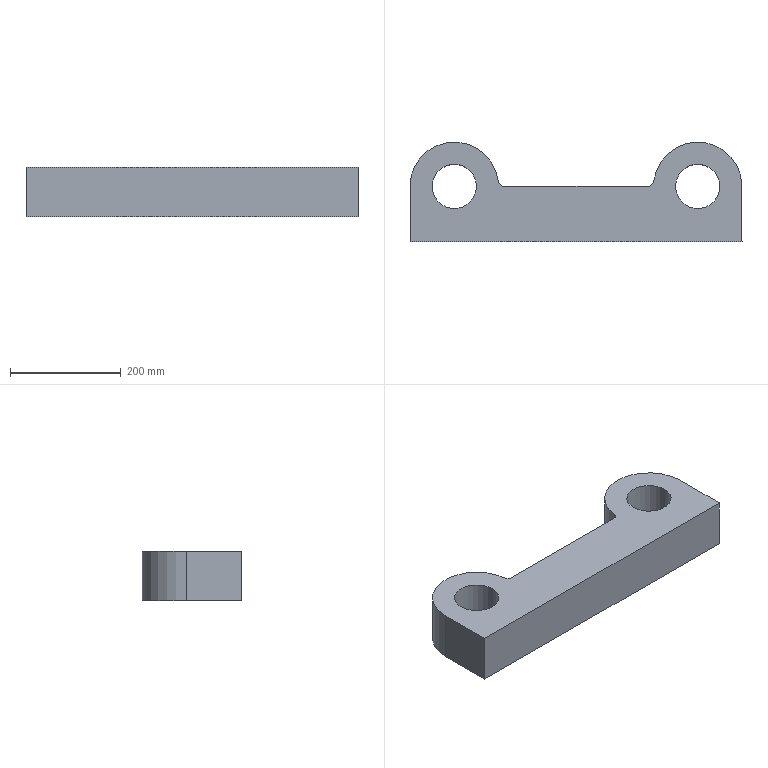Part | SolidWorks | features Extrusion 1 | 1 solid | 14 faces | box 600 x 180 x 90 mm | volume 6307881 mm3 | cylinder 8 | plane 6 | commonest cylinder face diameters 80 x4 20 x2 160 x2
STEP:
#1=CARTESIAN_POINT('',(260.,0.,90.));
#2=VERTEX_POINT('',#1);
#3=CARTESIAN_POINT('',(180.,0.,90.));
#4=VERTEX_POINT('',#3);
#5=CARTESIAN_POINT('',(220.,0.,90.));
#6=DIRECTION('',(0.,0.,-1.));
#7=DIRECTION('',(1.,0.,0.));
#8=AXIS2_PLACEMENT_3D('',#5,#6,#7);
#9=CIRCLE('',#8,40.);
#10=EDGE_CURVE('',#2,#4,#9,.T.);
#11=ORIENTED_EDGE('',*,*,#10,.F.);
#12=CARTESIAN_POINT('',(260.,0.,0.));
#13=VERTEX_POINT('',#12);
#14=CARTESIAN_POINT('',(260.,0.,90.));
#15=DIRECTION('',(0.,0.,-1.));
#16=VECTOR('',#15,1000.);
#17=LINE('',#14,#16);
#18=EDGE_CURVE('',#2,#13,#17,.T.);
#19=ORIENTED_EDGE('',*,*,#18,.T.);
#20=CARTESIAN_POINT('',(180.,0.,0.));
#21=VERTEX_POINT('',#20);
#22=CARTESIAN_POINT('',(220.,0.,0.));
#23=DIRECTION('',(0.,0.,-1.));
#24=DIRECTION('',(1.,0.,0.));
#25=AXIS2_PLACEMENT_3D('',#22,#23,#24);
#26=CIRCLE('',#25,40.);
#27=EDGE_CURVE('',#13,#21,#26,.T.);
#28=ORIENTED_EDGE('',*,*,#27,.T.);
#29=CARTESIAN_POINT('',(180.,0.,90.));
#30=DIRECTION('',(0.,0.,-1.));
#31=VECTOR('',#30,1000.);
#32=LINE('',#29,#31);
#33=EDGE_CURVE('',#4,#21,#32,.T.);
#34=ORIENTED_EDGE('',*,*,#33,.F.);
#35=EDGE_LOOP('',(#11,#19,#28,#34));
#36=FACE_OUTER_BOUND('',#35,.T.);
#37=CARTESIAN_POINT('',(220.,0.,90.));
#38=DIRECTION('',(0.,0.,-1.));
#39=DIRECTION('',(-1.,0.,0.));
#40=AXIS2_PLACEMENT_3D('',#37,#38,#39);
#41=CYLINDRICAL_SURFACE('',#40,40.);
#42=ADVANCED_FACE('',(#36),#41,.F.);
#43=CARTESIAN_POINT('',(-260.,0.,90.));
#44=VERTEX_POINT('',#43);
#45=CARTESIAN_POINT('',(-180.,0.,90.));
#46=VERTEX_POINT('',#45);
#47=CARTESIAN_POINT('',(-220.,0.,90.));
#48=DIRECTION('',(0.,0.,1.));
#49=DIRECTION('',(1.,0.,0.));
#50=AXIS2_PLACEMENT_3D('',#47,#48,#49);
#51=CIRCLE('',#50,40.);
#52=EDGE_CURVE('',#44,#46,#51,.T.);
#53=ORIENTED_EDGE('',*,*,#52,.T.);
#54=CARTESIAN_POINT('',(-180.,0.,0.));
#55=VERTEX_POINT('',#54);
#56=CARTESIAN_POINT('',(-180.,0.,90.));
#57=DIRECTION('',(0.,0.,-1.));
#58=VECTOR('',#57,1000.);
#59=LINE('',#56,#58);
#60=EDGE_CURVE('',#46,#55,#59,.T.);
#61=ORIENTED_EDGE('',*,*,#60,.T.);
#62=CARTESIAN_POINT('',(-260.,0.,0.));
#63=VERTEX_POINT('',#62);
#64=CARTESIAN_POINT('',(-220.,0.,0.));
#65=DIRECTION('',(0.,0.,1.));
#66=DIRECTION('',(1.,0.,0.));
#67=AXIS2_PLACEMENT_3D('',#64,#65,#66);
#68=CIRCLE('',#67,40.);
#69=EDGE_CURVE('',#63,#55,#68,.T.);
#70=ORIENTED_EDGE('',*,*,#69,.F.);
#71=CARTESIAN_POINT('',(-260.,0.,90.));
#72=DIRECTION('',(0.,0.,-1.));
#73=VECTOR('',#72,1000.);
#74=LINE('',#71,#73);
#75=EDGE_CURVE('',#44,#63,#74,.T.);
#76=ORIENTED_EDGE('',*,*,#75,.F.);
#77=EDGE_LOOP('',(#53,#61,#70,#76));
#78=FACE_OUTER_BOUND('',#77,.T.);
#79=CARTESIAN_POINT('',(-220.,0.,90.));
#80=DIRECTION('',(0.,0.,-1.));
#81=DIRECTION('',(-1.,0.,0.));
#82=AXIS2_PLACEMENT_3D('',#79,#80,#81);
#83=CYLINDRICAL_SURFACE('',#82,40.);
#84=ADVANCED_FACE('',(#78),#83,.F.);
#85=CARTESIAN_POINT('',(-130.557,0.,0.));
#86=VERTEX_POINT('',#85);
#87=CARTESIAN_POINT('',(130.557,0.,0.));
#88=VERTEX_POINT('',#87);
#89=CARTESIAN_POINT('',(0.,0.,0.));
#90=DIRECTION('',(1.,0.,0.));
#91=VECTOR('',#90,1000.);
#92=LINE('',#89,#91);
#93=EDGE_CURVE('',#86,#88,#92,.T.);
#94=ORIENTED_EDGE('',*,*,#93,.F.);
#95=CARTESIAN_POINT('',(-130.557,0.,90.));
#96=VERTEX_POINT('',#95);
#97=CARTESIAN_POINT('',(-130.557,0.,90.));
#98=DIRECTION('',(0.,0.,-1.));
#99=VECTOR('',#98,1000.);
#100=LINE('',#97,#99);
#101=EDGE_CURVE('',#96,#86,#100,.T.);
#102=ORIENTED_EDGE('',*,*,#101,.F.);
#103=CARTESIAN_POINT('',(130.557,0.,90.));
#104=VERTEX_POINT('',#103);
#105=CARTESIAN_POINT('',(0.,0.,90.));
#106=DIRECTION('',(1.,0.,0.));
#107=VECTOR('',#106,1000.);
#108=LINE('',#105,#107);
#109=EDGE_CURVE('',#96,#104,#108,.T.);
#110=ORIENTED_EDGE('',*,*,#109,.T.);
#111=CARTESIAN_POINT('',(130.557,0.,90.));
#112=DIRECTION('',(0.,0.,-1.));
#113=VECTOR('',#112,1000.);
#114=LINE('',#111,#113);
#115=EDGE_CURVE('',#104,#88,#114,.T.);
#116=ORIENTED_EDGE('',*,*,#115,.T.);
#117=EDGE_LOOP('',(#94,#102,#110,#116));
#118=FACE_OUTER_BOUND('',#117,.T.);
#119=CARTESIAN_POINT('',(0.,0.,90.));
#120=DIRECTION('',(0.,1.,0.));
#121=DIRECTION('',(0.,0.,1.));
#122=AXIS2_PLACEMENT_3D('',#119,#120,#121);
#123=PLANE('',#122);
#124=ADVANCED_FACE('',(#118),#123,.T.);
#125=CARTESIAN_POINT('',(-140.495,8.889,0.));
#126=VERTEX_POINT('',#125);
#127=CARTESIAN_POINT('',(-130.557,10.,0.));
#128=DIRECTION('',(0.,0.,-1.));
#129=DIRECTION('',(1.,0.,0.));
#130=AXIS2_PLACEMENT_3D('',#127,#128,#129);
#131=CIRCLE('',#130,10.);
#132=EDGE_CURVE('',#86,#126,#131,.T.);
#133=ORIENTED_EDGE('',*,*,#132,.T.);
#134=CARTESIAN_POINT('',(-140.495,8.889,90.));
#135=VERTEX_POINT('',#134);
#136=CARTESIAN_POINT('',(-140.495,8.889,90.));
#137=DIRECTION('',(0.,0.,-1.));
#138=VECTOR('',#137,1000.);
#139=LINE('',#136,#138);
#140=EDGE_CURVE('',#135,#126,#139,.T.);
#141=ORIENTED_EDGE('',*,*,#140,.F.);
#142=CARTESIAN_POINT('',(-130.557,10.,90.));
#143=DIRECTION('',(0.,0.,-1.));
#144=DIRECTION('',(1.,0.,0.));
#145=AXIS2_PLACEMENT_3D('',#142,#143,#144);
#146=CIRCLE('',#145,10.);
#147=EDGE_CURVE('',#96,#135,#146,.T.);
#148=ORIENTED_EDGE('',*,*,#147,.F.);
#149=ORIENTED_EDGE('',*,*,#101,.T.);
#150=EDGE_LOOP('',(#133,#141,#148,#149));
#151=FACE_OUTER_BOUND('',#150,.T.);
#152=CARTESIAN_POINT('',(-130.557,10.,90.));
#153=DIRECTION('',(0.,0.,-1.));
#154=DIRECTION('',(-1.,0.,0.));
#155=AXIS2_PLACEMENT_3D('',#152,#153,#154);
#156=CYLINDRICAL_SURFACE('',#155,10.);
#157=ADVANCED_FACE('',(#151),#156,.F.);
#158=CARTESIAN_POINT('',(-300.,0.,0.));
#159=VERTEX_POINT('',#158);
#160=CARTESIAN_POINT('',(-220.,0.,0.));
#161=DIRECTION('',(0.,0.,1.));
#162=DIRECTION('',(1.,0.,0.));
#163=AXIS2_PLACEMENT_3D('',#160,#161,#162);
#164=CIRCLE('',#163,80.);
#165=EDGE_CURVE('',#126,#159,#164,.T.);
#166=ORIENTED_EDGE('',*,*,#165,.T.);
#167=CARTESIAN_POINT('',(-300.,0.,90.));
#168=VERTEX_POINT('',#167);
#169=CARTESIAN_POINT('',(-300.,0.,90.));
#170=DIRECTION('',(0.,0.,-1.));
#171=VECTOR('',#170,1000.);
#172=LINE('',#169,#171);
#173=EDGE_CURVE('',#168,#159,#172,.T.);
#174=ORIENTED_EDGE('',*,*,#173,.F.);
#175=CARTESIAN_POINT('',(-220.,0.,90.));
#176=DIRECTION('',(0.,0.,1.));
#177=DIRECTION('',(1.,0.,0.));
#178=AXIS2_PLACEMENT_3D('',#175,#176,#177);
#179=CIRCLE('',#178,80.);
#180=EDGE_CURVE('',#135,#168,#179,.T.);
#181=ORIENTED_EDGE('',*,*,#180,.F.);
#182=ORIENTED_EDGE('',*,*,#140,.T.);
#183=EDGE_LOOP('',(#166,#174,#181,#182));
#184=FACE_OUTER_BOUND('',#183,.T.);
#185=CARTESIAN_POINT('',(-220.,0.,90.));
#186=DIRECTION('',(0.,0.,-1.));
#187=DIRECTION('',(-1.,0.,0.));
#188=AXIS2_PLACEMENT_3D('',#185,#186,#187);
#189=CYLINDRICAL_SURFACE('',#188,80.);
#190=ADVANCED_FACE('',(#184),#189,.T.);
#191=CARTESIAN_POINT('',(-300.,-100.,0.));
#192=VERTEX_POINT('',#191);
#193=CARTESIAN_POINT('',(-300.,0.,0.));
#194=DIRECTION('',(0.,-1.,0.));
#195=VECTOR('',#194,1000.);
#196=LINE('',#193,#195);
#197=EDGE_CURVE('',#159,#192,#196,.T.);
#198=ORIENTED_EDGE('',*,*,#197,.T.);
#199=CARTESIAN_POINT('',(-300.,-100.,90.));
#200=VERTEX_POINT('',#199);
#201=CARTESIAN_POINT('',(-300.,-100.,90.));
#202=DIRECTION('',(0.,0.,-1.));
#203=VECTOR('',#202,1000.);
#204=LINE('',#201,#203);
#205=EDGE_CURVE('',#200,#192,#204,.T.);
#206=ORIENTED_EDGE('',*,*,#205,.F.);
#207=CARTESIAN_POINT('',(-300.,0.,90.));
#208=DIRECTION('',(0.,-1.,0.));
#209=VECTOR('',#208,1000.);
#210=LINE('',#207,#209);
#211=EDGE_CURVE('',#168,#200,#210,.T.);
#212=ORIENTED_EDGE('',*,*,#211,.F.);
#213=ORIENTED_EDGE('',*,*,#173,.T.);
#214=EDGE_LOOP('',(#198,#206,#212,#213));
#215=FACE_OUTER_BOUND('',#214,.T.);
#216=CARTESIAN_POINT('',(-300.,0.,90.));
#217=DIRECTION('',(1.,0.,0.));
#218=DIRECTION('',(0.,0.,-1.));
#219=AXIS2_PLACEMENT_3D('',#216,#217,#218);
#220=PLANE('',#219);
#221=ADVANCED_FACE('',(#215),#220,.F.);
#222=CARTESIAN_POINT('',(300.,-100.,0.));
#223=VERTEX_POINT('',#222);
#224=CARTESIAN_POINT('',(0.,-100.,0.));
#225=DIRECTION('',(1.,0.,0.));
#226=VECTOR('',#225,1000.);
#227=LINE('',#224,#226);
#228=EDGE_CURVE('',#192,#223,#227,.T.);
#229=ORIENTED_EDGE('',*,*,#228,.T.);
#230=CARTESIAN_POINT('',(300.,-100.,90.));
#231=VERTEX_POINT('',#230);
#232=CARTESIAN_POINT('',(300.,-100.,90.));
#233=DIRECTION('',(0.,0.,-1.));
#234=VECTOR('',#233,1000.);
#235=LINE('',#232,#234);
#236=EDGE_CURVE('',#231,#223,#235,.T.);
#237=ORIENTED_EDGE('',*,*,#236,.F.);
#238=CARTESIAN_POINT('',(0.,-100.,90.));
#239=DIRECTION('',(1.,0.,0.));
#240=VECTOR('',#239,1000.);
#241=LINE('',#238,#240);
#242=EDGE_CURVE('',#200,#231,#241,.T.);
#243=ORIENTED_EDGE('',*,*,#242,.F.);
#244=ORIENTED_EDGE('',*,*,#205,.T.);
#245=EDGE_LOOP('',(#229,#237,#243,#244));
#246=FACE_OUTER_BOUND('',#245,.T.);
#247=CARTESIAN_POINT('',(0.,-100.,90.));
#248=DIRECTION('',(0.,1.,0.));
#249=DIRECTION('',(0.,0.,1.));
#250=AXIS2_PLACEMENT_3D('',#247,#248,#249);
#251=PLANE('',#250);
#252=ADVANCED_FACE('',(#246),#251,.F.);
#253=CARTESIAN_POINT('',(299.972,2.127,0.));
#254=VERTEX_POINT('',#253);
#255=CARTESIAN_POINT('',(299.972,0.08308,0.));
#256=DIRECTION('',(-0.0002769,1.,0.));
#257=VECTOR('',#256,1000.);
#258=LINE('',#255,#257);
#259=EDGE_CURVE('',#223,#254,#258,.T.);
#260=ORIENTED_EDGE('',*,*,#259,.T.);
#261=CARTESIAN_POINT('',(299.972,2.127,90.));
#262=VERTEX_POINT('',#261);
#263=CARTESIAN_POINT('',(299.972,2.127,90.));
#264=DIRECTION('',(0.,0.,-1.));
#265=VECTOR('',#264,1000.);
#266=LINE('',#263,#265);
#267=EDGE_CURVE('',#262,#254,#266,.T.);
#268=ORIENTED_EDGE('',*,*,#267,.F.);
#269=CARTESIAN_POINT('',(299.972,0.08308,90.));
#270=DIRECTION('',(-0.0002769,1.,0.));
#271=VECTOR('',#270,1000.);
#272=LINE('',#269,#271);
#273=EDGE_CURVE('',#231,#262,#272,.T.);
#274=ORIENTED_EDGE('',*,*,#273,.F.);
#275=ORIENTED_EDGE('',*,*,#236,.T.);
#276=EDGE_LOOP('',(#260,#268,#274,#275));
#277=FACE_OUTER_BOUND('',#276,.T.);
#278=CARTESIAN_POINT('',(299.972,0.08308,90.));
#279=DIRECTION('',(-1.,-0.0002769,0.));
#280=DIRECTION('',(0.0002769,-1.,0.));
#281=AXIS2_PLACEMENT_3D('',#278,#279,#280);
#282=PLANE('',#281);
#283=ADVANCED_FACE('',(#277),#282,.F.);
#284=CARTESIAN_POINT('',(140.495,8.889,0.));
#285=VERTEX_POINT('',#284);
#286=CARTESIAN_POINT('',(220.,0.,0.));
#287=DIRECTION('',(0.,0.,1.));
#288=DIRECTION('',(1.,0.,0.));
#289=AXIS2_PLACEMENT_3D('',#286,#287,#288);
#290=CIRCLE('',#289,80.);
#291=EDGE_CURVE('',#254,#285,#290,.T.);
#292=ORIENTED_EDGE('',*,*,#291,.T.);
#293=CARTESIAN_POINT('',(140.495,8.889,90.));
#294=VERTEX_POINT('',#293);
#295=CARTESIAN_POINT('',(140.495,8.889,90.));
#296=DIRECTION('',(0.,0.,-1.));
#297=VECTOR('',#296,1000.);
#298=LINE('',#295,#297);
#299=EDGE_CURVE('',#294,#285,#298,.T.);
#300=ORIENTED_EDGE('',*,*,#299,.F.);
#301=CARTESIAN_POINT('',(220.,0.,90.));
#302=DIRECTION('',(0.,0.,1.));
#303=DIRECTION('',(1.,0.,0.));
#304=AXIS2_PLACEMENT_3D('',#301,#302,#303);
#305=CIRCLE('',#304,80.);
#306=EDGE_CURVE('',#262,#294,#305,.T.);
#307=ORIENTED_EDGE('',*,*,#306,.F.);
#308=ORIENTED_EDGE('',*,*,#267,.T.);
#309=EDGE_LOOP('',(#292,#300,#307,#308));
#310=FACE_OUTER_BOUND('',#309,.T.);
#311=CARTESIAN_POINT('',(220.,0.,90.));
#312=DIRECTION('',(0.,0.,-1.));
#313=DIRECTION('',(-1.,0.,0.));
#314=AXIS2_PLACEMENT_3D('',#311,#312,#313);
#315=CYLINDRICAL_SURFACE('',#314,80.);
#316=ADVANCED_FACE('',(#310),#315,.T.);
#317=ORIENTED_EDGE('',*,*,#60,.F.);
#318=CARTESIAN_POINT('',(-220.,0.,90.));
#319=DIRECTION('',(0.,0.,1.));
#320=DIRECTION('',(1.,0.,0.));
#321=AXIS2_PLACEMENT_3D('',#318,#319,#320);
#322=CIRCLE('',#321,40.);
#323=EDGE_CURVE('',#46,#44,#322,.T.);
#324=ORIENTED_EDGE('',*,*,#323,.T.);
#325=ORIENTED_EDGE('',*,*,#75,.T.);
#326=CARTESIAN_POINT('',(-220.,0.,0.));
#327=DIRECTION('',(0.,0.,1.));
#328=DIRECTION('',(1.,0.,0.));
#329=AXIS2_PLACEMENT_3D('',#326,#327,#328);
#330=CIRCLE('',#329,40.);
#331=EDGE_CURVE('',#55,#63,#330,.T.);
#332=ORIENTED_EDGE('',*,*,#331,.F.);
#333=EDGE_LOOP('',(#317,#324,#325,#332));
#334=FACE_OUTER_BOUND('',#333,.T.);
#335=CARTESIAN_POINT('',(-220.,0.,90.));
#336=DIRECTION('',(0.,0.,-1.));
#337=DIRECTION('',(-1.,0.,0.));
#338=AXIS2_PLACEMENT_3D('',#335,#336,#337);
#339=CYLINDRICAL_SURFACE('',#338,40.);
#340=ADVANCED_FACE('',(#334),#339,.F.);
#341=ORIENTED_EDGE('',*,*,#18,.F.);
#342=CARTESIAN_POINT('',(220.,0.,90.));
#343=DIRECTION('',(0.,0.,-1.));
#344=DIRECTION('',(1.,0.,0.));
#345=AXIS2_PLACEMENT_3D('',#342,#343,#344);
#346=CIRCLE('',#345,40.);
#347=EDGE_CURVE('',#4,#2,#346,.T.);
#348=ORIENTED_EDGE('',*,*,#347,.F.);
#349=ORIENTED_EDGE('',*,*,#33,.T.);
#350=CARTESIAN_POINT('',(220.,0.,0.));
#351=DIRECTION('',(0.,0.,-1.));
#352=DIRECTION('',(1.,0.,0.));
#353=AXIS2_PLACEMENT_3D('',#350,#351,#352);
#354=CIRCLE('',#353,40.);
#355=EDGE_CURVE('',#21,#13,#354,.T.);
#356=ORIENTED_EDGE('',*,*,#355,.T.);
#357=EDGE_LOOP('',(#341,#348,#349,#356));
#358=FACE_OUTER_BOUND('',#357,.T.);
#359=CARTESIAN_POINT('',(220.,0.,90.));
#360=DIRECTION('',(0.,0.,-1.));
#361=DIRECTION('',(-1.,0.,0.));
#362=AXIS2_PLACEMENT_3D('',#359,#360,#361);
#363=CYLINDRICAL_SURFACE('',#362,40.);
#364=ADVANCED_FACE('',(#358),#363,.F.);
#365=CARTESIAN_POINT('',(130.557,10.,0.));
#366=DIRECTION('',(0.,0.,1.));
#367=DIRECTION('',(1.,0.,0.));
#368=AXIS2_PLACEMENT_3D('',#365,#366,#367);
#369=CIRCLE('',#368,10.);
#370=EDGE_CURVE('',#88,#285,#369,.T.);
#371=ORIENTED_EDGE('',*,*,#370,.F.);
#372=ORIENTED_EDGE('',*,*,#115,.F.);
#373=CARTESIAN_POINT('',(130.557,10.,90.));
#374=DIRECTION('',(0.,0.,1.));
#375=DIRECTION('',(1.,0.,0.));
#376=AXIS2_PLACEMENT_3D('',#373,#374,#375);
#377=CIRCLE('',#376,10.);
#378=EDGE_CURVE('',#104,#294,#377,.T.);
#379=ORIENTED_EDGE('',*,*,#378,.T.);
#380=ORIENTED_EDGE('',*,*,#299,.T.);
#381=EDGE_LOOP('',(#371,#372,#379,#380));
#382=FACE_OUTER_BOUND('',#381,.T.);
#383=CARTESIAN_POINT('',(130.557,10.,90.));
#384=DIRECTION('',(0.,0.,-1.));
#385=DIRECTION('',(-1.,0.,0.));
#386=AXIS2_PLACEMENT_3D('',#383,#384,#385);
#387=CYLINDRICAL_SURFACE('',#386,10.);
#388=ADVANCED_FACE('',(#382),#387,.F.);
#389=ORIENTED_EDGE('',*,*,#347,.T.);
#390=ORIENTED_EDGE('',*,*,#10,.T.);
#391=EDGE_LOOP('',(#389,#390));
#392=FACE_BOUND('',#391,.T.);
#393=ORIENTED_EDGE('',*,*,#52,.F.);
#394=ORIENTED_EDGE('',*,*,#323,.F.);
#395=EDGE_LOOP('',(#393,#394));
#396=FACE_BOUND('',#395,.T.);
#397=ORIENTED_EDGE('',*,*,#109,.F.);
#398=ORIENTED_EDGE('',*,*,#147,.T.);
#399=ORIENTED_EDGE('',*,*,#180,.T.);
#400=ORIENTED_EDGE('',*,*,#211,.T.);
#401=ORIENTED_EDGE('',*,*,#242,.T.);
#402=ORIENTED_EDGE('',*,*,#273,.T.);
#403=ORIENTED_EDGE('',*,*,#306,.T.);
#404=ORIENTED_EDGE('',*,*,#378,.F.);
#405=EDGE_LOOP('',(#397,#398,#399,#400,#401,#402,#403,#404));
#406=FACE_OUTER_BOUND('',#405,.T.);
#407=CARTESIAN_POINT('',(0.,0.,90.));
#408=DIRECTION('',(0.,0.,1.));
#409=DIRECTION('',(1.,0.,0.));
#410=AXIS2_PLACEMENT_3D('',#407,#408,#409);
#411=PLANE('',#410);
#412=ADVANCED_FACE('',(#392,#396,#406),#411,.T.);
#413=ORIENTED_EDGE('',*,*,#355,.F.);
#414=ORIENTED_EDGE('',*,*,#27,.F.);
#415=EDGE_LOOP('',(#413,#414));
#416=FACE_BOUND('',#415,.T.);
#417=ORIENTED_EDGE('',*,*,#69,.T.);
#418=ORIENTED_EDGE('',*,*,#331,.T.);
#419=EDGE_LOOP('',(#417,#418));
#420=FACE_BOUND('',#419,.T.);
#421=ORIENTED_EDGE('',*,*,#93,.T.);
#422=ORIENTED_EDGE('',*,*,#370,.T.);
#423=ORIENTED_EDGE('',*,*,#291,.F.);
#424=ORIENTED_EDGE('',*,*,#259,.F.);
#425=ORIENTED_EDGE('',*,*,#228,.F.);
#426=ORIENTED_EDGE('',*,*,#197,.F.);
#427=ORIENTED_EDGE('',*,*,#165,.F.);
#428=ORIENTED_EDGE('',*,*,#132,.F.);
#429=EDGE_LOOP('',(#421,#422,#423,#424,#425,#426,#427,#428));
#430=FACE_OUTER_BOUND('',#429,.T.);
#431=CARTESIAN_POINT('',(0.,0.,0.));
#432=DIRECTION('',(0.,0.,1.));
#433=DIRECTION('',(1.,0.,0.));
#434=AXIS2_PLACEMENT_3D('',#431,#432,#433);
#435=PLANE('',#434);
#436=ADVANCED_FACE('',(#416,#420,#430),#435,.F.);
#437=CLOSED_SHELL('',(#42,#84,#124,#157,#190,#221,#252,#283,#316,#340,#364,#388,#412,#436));
#438=MANIFOLD_SOLID_BREP('',#437);
#439=CARTESIAN_POINT('',(0.,0.,0.));
#440=DIRECTION('',(0.,0.,1.));
#441=DIRECTION('',(1.,0.,0.));
#442=AXIS2_PLACEMENT_3D('',#439,#440,#441);
#443=(LENGTH_UNIT()NAMED_UNIT(*)SI_UNIT(.MILLI.,.METRE.));
#444=UNCERTAINTY_MEASURE_WITH_UNIT(LENGTH_MEASURE(0.00001),#443,'','');
#445=(NAMED_UNIT(*)PLANE_ANGLE_UNIT()SI_UNIT($,.RADIAN.));
#446=(NAMED_UNIT(*)SI_UNIT($,.STERADIAN.)SOLID_ANGLE_UNIT());
#447=(GEOMETRIC_REPRESENTATION_CONTEXT(3)GLOBAL_UNCERTAINTY_ASSIGNED_CONTEXT((#444))GLOBAL_UNIT_ASSIGNED_CONTEXT((#443,#445,#446))REPRESENTATION_CONTEXT('',''));
#448=ADVANCED_BREP_SHAPE_REPRESENTATION('',(#438,#442),#447);